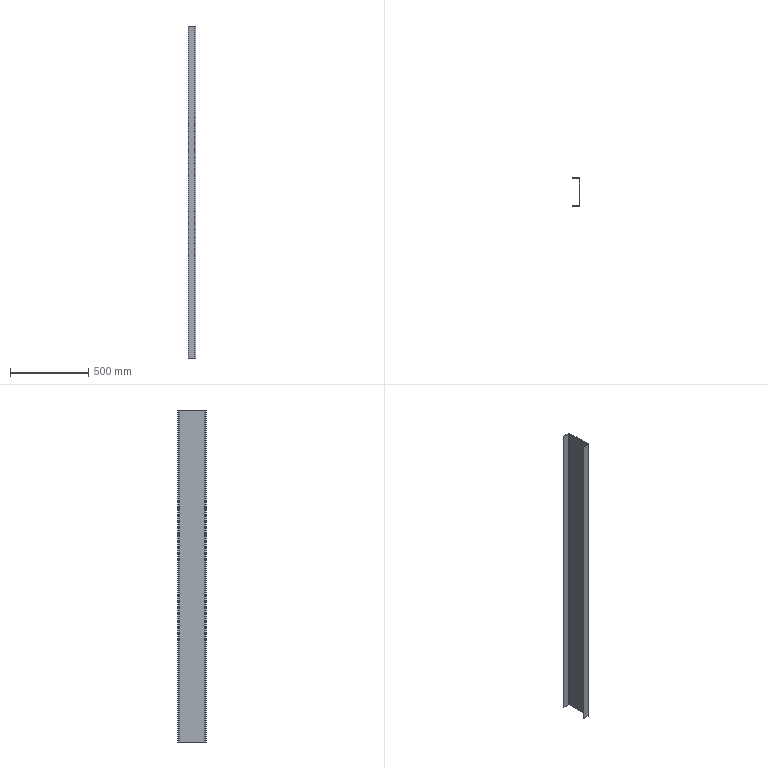Part | SolidWorks | features Extrusion 1 | 1 solid | 14 faces | box 50 x 180 x 2124 mm | volume 2267154 mm3 | plane 10 | cylinder 4 | commonest cylinder face diameters 8 x2 16 x2
STEP:
#1=CARTESIAN_POINT('',(-50.,-86.,-1062.));
#2=VERTEX_POINT('',#1);
#3=CARTESIAN_POINT('',(-50.,-90.,-1062.));
#4=VERTEX_POINT('',#3);
#5=CARTESIAN_POINT('',(-50.,-86.,-1062.));
#6=DIRECTION('',(0.,-1.,0.));
#7=VECTOR('',#6,1000.);
#8=LINE('',#5,#7);
#9=EDGE_CURVE('',#2,#4,#8,.T.);
#10=ORIENTED_EDGE('',*,*,#9,.T.);
#11=CARTESIAN_POINT('',(-50.,-90.,1062.));
#12=VERTEX_POINT('',#11);
#13=CARTESIAN_POINT('',(-50.,-90.,1062.));
#14=DIRECTION('',(0.,0.,-1.));
#15=VECTOR('',#14,1000.);
#16=LINE('',#13,#15);
#17=EDGE_CURVE('',#12,#4,#16,.T.);
#18=ORIENTED_EDGE('',*,*,#17,.F.);
#19=CARTESIAN_POINT('',(-50.,-86.,1062.));
#20=VERTEX_POINT('',#19);
#21=CARTESIAN_POINT('',(-50.,-86.,1062.));
#22=DIRECTION('',(0.,-1.,0.));
#23=VECTOR('',#22,1000.);
#24=LINE('',#21,#23);
#25=EDGE_CURVE('',#20,#12,#24,.T.);
#26=ORIENTED_EDGE('',*,*,#25,.F.);
#27=CARTESIAN_POINT('',(-50.,-86.,1062.));
#28=DIRECTION('',(0.,0.,-1.));
#29=VECTOR('',#28,1000.);
#30=LINE('',#27,#29);
#31=EDGE_CURVE('',#20,#2,#30,.T.);
#32=ORIENTED_EDGE('',*,*,#31,.T.);
#33=EDGE_LOOP('',(#10,#18,#26,#32));
#34=FACE_OUTER_BOUND('',#33,.T.);
#35=CARTESIAN_POINT('',(-50.,-86.,1062.));
#36=DIRECTION('',(1.,0.,0.));
#37=DIRECTION('',(0.,0.,-1.));
#38=AXIS2_PLACEMENT_3D('',#35,#36,#37);
#39=PLANE('',#38);
#40=ADVANCED_FACE('',(#34),#39,.F.);
#41=CARTESIAN_POINT('',(-8.,-90.,-1062.));
#42=VERTEX_POINT('',#41);
#43=CARTESIAN_POINT('',(-50.,-90.,-1062.));
#44=DIRECTION('',(1.,0.,0.));
#45=VECTOR('',#44,1000.);
#46=LINE('',#43,#45);
#47=EDGE_CURVE('',#4,#42,#46,.T.);
#48=ORIENTED_EDGE('',*,*,#47,.T.);
#49=CARTESIAN_POINT('',(-8.,-90.,1062.));
#50=VERTEX_POINT('',#49);
#51=CARTESIAN_POINT('',(-8.,-90.,1062.));
#52=DIRECTION('',(0.,0.,-1.));
#53=VECTOR('',#52,1000.);
#54=LINE('',#51,#53);
#55=EDGE_CURVE('',#50,#42,#54,.T.);
#56=ORIENTED_EDGE('',*,*,#55,.F.);
#57=CARTESIAN_POINT('',(-50.,-90.,1062.));
#58=DIRECTION('',(1.,0.,0.));
#59=VECTOR('',#58,1000.);
#60=LINE('',#57,#59);
#61=EDGE_CURVE('',#12,#50,#60,.T.);
#62=ORIENTED_EDGE('',*,*,#61,.F.);
#63=ORIENTED_EDGE('',*,*,#17,.T.);
#64=EDGE_LOOP('',(#48,#56,#62,#63));
#65=FACE_OUTER_BOUND('',#64,.T.);
#66=CARTESIAN_POINT('',(-50.,-90.,1062.));
#67=DIRECTION('',(0.,1.,0.));
#68=DIRECTION('',(0.,0.,1.));
#69=AXIS2_PLACEMENT_3D('',#66,#67,#68);
#70=PLANE('',#69);
#71=ADVANCED_FACE('',(#65),#70,.F.);
#72=CARTESIAN_POINT('',(0.,-82.,-1062.));
#73=VERTEX_POINT('',#72);
#74=CARTESIAN_POINT('',(-8.,-82.,-1062.));
#75=DIRECTION('',(0.,0.,1.));
#76=DIRECTION('',(1.,0.,0.));
#77=AXIS2_PLACEMENT_3D('',#74,#75,#76);
#78=CIRCLE('',#77,8.);
#79=EDGE_CURVE('',#42,#73,#78,.T.);
#80=ORIENTED_EDGE('',*,*,#79,.T.);
#81=CARTESIAN_POINT('',(0.,-82.,1062.));
#82=VERTEX_POINT('',#81);
#83=CARTESIAN_POINT('',(0.,-82.,1062.));
#84=DIRECTION('',(0.,0.,-1.));
#85=VECTOR('',#84,1000.);
#86=LINE('',#83,#85);
#87=EDGE_CURVE('',#82,#73,#86,.T.);
#88=ORIENTED_EDGE('',*,*,#87,.F.);
#89=CARTESIAN_POINT('',(-8.,-82.,1062.));
#90=DIRECTION('',(0.,0.,1.));
#91=DIRECTION('',(1.,0.,0.));
#92=AXIS2_PLACEMENT_3D('',#89,#90,#91);
#93=CIRCLE('',#92,8.);
#94=EDGE_CURVE('',#50,#82,#93,.T.);
#95=ORIENTED_EDGE('',*,*,#94,.F.);
#96=ORIENTED_EDGE('',*,*,#55,.T.);
#97=EDGE_LOOP('',(#80,#88,#95,#96));
#98=FACE_OUTER_BOUND('',#97,.T.);
#99=CARTESIAN_POINT('',(-8.,-82.,1062.));
#100=DIRECTION('',(0.,0.,-1.));
#101=DIRECTION('',(-1.,0.,0.));
#102=AXIS2_PLACEMENT_3D('',#99,#100,#101);
#103=CYLINDRICAL_SURFACE('',#102,8.);
#104=ADVANCED_FACE('',(#98),#103,.T.);
#105=CARTESIAN_POINT('',(0.,82.,-1062.));
#106=VERTEX_POINT('',#105);
#107=CARTESIAN_POINT('',(0.,-82.,-1062.));
#108=DIRECTION('',(0.,1.,0.));
#109=VECTOR('',#108,1000.);
#110=LINE('',#107,#109);
#111=EDGE_CURVE('',#73,#106,#110,.T.);
#112=ORIENTED_EDGE('',*,*,#111,.T.);
#113=CARTESIAN_POINT('',(0.,82.,1062.));
#114=VERTEX_POINT('',#113);
#115=CARTESIAN_POINT('',(0.,82.,1062.));
#116=DIRECTION('',(0.,0.,-1.));
#117=VECTOR('',#116,1000.);
#118=LINE('',#115,#117);
#119=EDGE_CURVE('',#114,#106,#118,.T.);
#120=ORIENTED_EDGE('',*,*,#119,.F.);
#121=CARTESIAN_POINT('',(0.,-82.,1062.));
#122=DIRECTION('',(0.,1.,0.));
#123=VECTOR('',#122,1000.);
#124=LINE('',#121,#123);
#125=EDGE_CURVE('',#82,#114,#124,.T.);
#126=ORIENTED_EDGE('',*,*,#125,.F.);
#127=ORIENTED_EDGE('',*,*,#87,.T.);
#128=EDGE_LOOP('',(#112,#120,#126,#127));
#129=FACE_OUTER_BOUND('',#128,.T.);
#130=CARTESIAN_POINT('',(0.,-82.,1062.));
#131=DIRECTION('',(-1.,0.,0.));
#132=DIRECTION('',(0.,0.,1.));
#133=AXIS2_PLACEMENT_3D('',#130,#131,#132);
#134=PLANE('',#133);
#135=ADVANCED_FACE('',(#129),#134,.F.);
#136=CARTESIAN_POINT('',(-8.,90.,-1062.));
#137=VERTEX_POINT('',#136);
#138=CARTESIAN_POINT('',(-8.,82.,-1062.));
#139=DIRECTION('',(0.,0.,1.));
#140=DIRECTION('',(1.,0.,0.));
#141=AXIS2_PLACEMENT_3D('',#138,#139,#140);
#142=CIRCLE('',#141,8.);
#143=EDGE_CURVE('',#106,#137,#142,.T.);
#144=ORIENTED_EDGE('',*,*,#143,.T.);
#145=CARTESIAN_POINT('',(-8.,90.,1062.));
#146=VERTEX_POINT('',#145);
#147=CARTESIAN_POINT('',(-8.,90.,1062.));
#148=DIRECTION('',(0.,0.,-1.));
#149=VECTOR('',#148,1000.);
#150=LINE('',#147,#149);
#151=EDGE_CURVE('',#146,#137,#150,.T.);
#152=ORIENTED_EDGE('',*,*,#151,.F.);
#153=CARTESIAN_POINT('',(-8.,82.,1062.));
#154=DIRECTION('',(0.,0.,1.));
#155=DIRECTION('',(1.,0.,0.));
#156=AXIS2_PLACEMENT_3D('',#153,#154,#155);
#157=CIRCLE('',#156,8.);
#158=EDGE_CURVE('',#114,#146,#157,.T.);
#159=ORIENTED_EDGE('',*,*,#158,.F.);
#160=ORIENTED_EDGE('',*,*,#119,.T.);
#161=EDGE_LOOP('',(#144,#152,#159,#160));
#162=FACE_OUTER_BOUND('',#161,.T.);
#163=CARTESIAN_POINT('',(-8.,82.,1062.));
#164=DIRECTION('',(0.,0.,-1.));
#165=DIRECTION('',(-1.,0.,0.));
#166=AXIS2_PLACEMENT_3D('',#163,#164,#165);
#167=CYLINDRICAL_SURFACE('',#166,8.);
#168=ADVANCED_FACE('',(#162),#167,.T.);
#169=CARTESIAN_POINT('',(-50.,90.,-1062.));
#170=VERTEX_POINT('',#169);
#171=CARTESIAN_POINT('',(-8.,90.,-1062.));
#172=DIRECTION('',(-1.,0.,0.));
#173=VECTOR('',#172,1000.);
#174=LINE('',#171,#173);
#175=EDGE_CURVE('',#137,#170,#174,.T.);
#176=ORIENTED_EDGE('',*,*,#175,.T.);
#177=CARTESIAN_POINT('',(-50.,90.,1062.));
#178=VERTEX_POINT('',#177);
#179=CARTESIAN_POINT('',(-50.,90.,1062.));
#180=DIRECTION('',(0.,0.,-1.));
#181=VECTOR('',#180,1000.);
#182=LINE('',#179,#181);
#183=EDGE_CURVE('',#178,#170,#182,.T.);
#184=ORIENTED_EDGE('',*,*,#183,.F.);
#185=CARTESIAN_POINT('',(-8.,90.,1062.));
#186=DIRECTION('',(-1.,0.,0.));
#187=VECTOR('',#186,1000.);
#188=LINE('',#185,#187);
#189=EDGE_CURVE('',#146,#178,#188,.T.);
#190=ORIENTED_EDGE('',*,*,#189,.F.);
#191=ORIENTED_EDGE('',*,*,#151,.T.);
#192=EDGE_LOOP('',(#176,#184,#190,#191));
#193=FACE_OUTER_BOUND('',#192,.T.);
#194=CARTESIAN_POINT('',(-8.,90.,1062.));
#195=DIRECTION('',(0.,-1.,0.));
#196=DIRECTION('',(0.,0.,-1.));
#197=AXIS2_PLACEMENT_3D('',#194,#195,#196);
#198=PLANE('',#197);
#199=ADVANCED_FACE('',(#193),#198,.F.);
#200=CARTESIAN_POINT('',(-50.,86.,-1062.));
#201=VERTEX_POINT('',#200);
#202=CARTESIAN_POINT('',(-50.,90.,-1062.));
#203=DIRECTION('',(0.,-1.,0.));
#204=VECTOR('',#203,1000.);
#205=LINE('',#202,#204);
#206=EDGE_CURVE('',#170,#201,#205,.T.);
#207=ORIENTED_EDGE('',*,*,#206,.T.);
#208=CARTESIAN_POINT('',(-50.,86.,1062.));
#209=VERTEX_POINT('',#208);
#210=CARTESIAN_POINT('',(-50.,86.,1062.));
#211=DIRECTION('',(0.,0.,-1.));
#212=VECTOR('',#211,1000.);
#213=LINE('',#210,#212);
#214=EDGE_CURVE('',#209,#201,#213,.T.);
#215=ORIENTED_EDGE('',*,*,#214,.F.);
#216=CARTESIAN_POINT('',(-50.,90.,1062.));
#217=DIRECTION('',(0.,-1.,0.));
#218=VECTOR('',#217,1000.);
#219=LINE('',#216,#218);
#220=EDGE_CURVE('',#178,#209,#219,.T.);
#221=ORIENTED_EDGE('',*,*,#220,.F.);
#222=ORIENTED_EDGE('',*,*,#183,.T.);
#223=EDGE_LOOP('',(#207,#215,#221,#222));
#224=FACE_OUTER_BOUND('',#223,.T.);
#225=CARTESIAN_POINT('',(-50.,90.,1062.));
#226=DIRECTION('',(1.,0.,0.));
#227=DIRECTION('',(0.,0.,-1.));
#228=AXIS2_PLACEMENT_3D('',#225,#226,#227);
#229=PLANE('',#228);
#230=ADVANCED_FACE('',(#224),#229,.F.);
#231=CARTESIAN_POINT('',(-8.,86.,-1062.));
#232=VERTEX_POINT('',#231);
#233=CARTESIAN_POINT('',(-50.,86.,-1062.));
#234=DIRECTION('',(1.,0.,0.));
#235=VECTOR('',#234,1000.);
#236=LINE('',#233,#235);
#237=EDGE_CURVE('',#201,#232,#236,.T.);
#238=ORIENTED_EDGE('',*,*,#237,.T.);
#239=CARTESIAN_POINT('',(-8.,86.,1062.));
#240=VERTEX_POINT('',#239);
#241=CARTESIAN_POINT('',(-8.,86.,1062.));
#242=DIRECTION('',(0.,0.,-1.));
#243=VECTOR('',#242,1000.);
#244=LINE('',#241,#243);
#245=EDGE_CURVE('',#240,#232,#244,.T.);
#246=ORIENTED_EDGE('',*,*,#245,.F.);
#247=CARTESIAN_POINT('',(-50.,86.,1062.));
#248=DIRECTION('',(1.,0.,0.));
#249=VECTOR('',#248,1000.);
#250=LINE('',#247,#249);
#251=EDGE_CURVE('',#209,#240,#250,.T.);
#252=ORIENTED_EDGE('',*,*,#251,.F.);
#253=ORIENTED_EDGE('',*,*,#214,.T.);
#254=EDGE_LOOP('',(#238,#246,#252,#253));
#255=FACE_OUTER_BOUND('',#254,.T.);
#256=CARTESIAN_POINT('',(-50.,86.,1062.));
#257=DIRECTION('',(0.,1.,0.));
#258=DIRECTION('',(0.,0.,1.));
#259=AXIS2_PLACEMENT_3D('',#256,#257,#258);
#260=PLANE('',#259);
#261=ADVANCED_FACE('',(#255),#260,.F.);
#262=CARTESIAN_POINT('',(-4.,82.,-1062.));
#263=VERTEX_POINT('',#262);
#264=CARTESIAN_POINT('',(-8.,82.,-1062.));
#265=DIRECTION('',(0.,0.,-1.));
#266=DIRECTION('',(1.,0.,0.));
#267=AXIS2_PLACEMENT_3D('',#264,#265,#266);
#268=CIRCLE('',#267,4.);
#269=EDGE_CURVE('',#232,#263,#268,.T.);
#270=ORIENTED_EDGE('',*,*,#269,.T.);
#271=CARTESIAN_POINT('',(-4.,82.,1062.));
#272=VERTEX_POINT('',#271);
#273=CARTESIAN_POINT('',(-4.,82.,1062.));
#274=DIRECTION('',(0.,0.,-1.));
#275=VECTOR('',#274,1000.);
#276=LINE('',#273,#275);
#277=EDGE_CURVE('',#272,#263,#276,.T.);
#278=ORIENTED_EDGE('',*,*,#277,.F.);
#279=CARTESIAN_POINT('',(-8.,82.,1062.));
#280=DIRECTION('',(0.,0.,-1.));
#281=DIRECTION('',(1.,0.,0.));
#282=AXIS2_PLACEMENT_3D('',#279,#280,#281);
#283=CIRCLE('',#282,4.);
#284=EDGE_CURVE('',#240,#272,#283,.T.);
#285=ORIENTED_EDGE('',*,*,#284,.F.);
#286=ORIENTED_EDGE('',*,*,#245,.T.);
#287=EDGE_LOOP('',(#270,#278,#285,#286));
#288=FACE_OUTER_BOUND('',#287,.T.);
#289=CARTESIAN_POINT('',(-8.,82.,1062.));
#290=DIRECTION('',(0.,0.,-1.));
#291=DIRECTION('',(-1.,0.,0.));
#292=AXIS2_PLACEMENT_3D('',#289,#290,#291);
#293=CYLINDRICAL_SURFACE('',#292,4.);
#294=ADVANCED_FACE('',(#288),#293,.F.);
#295=CARTESIAN_POINT('',(-4.,-82.,-1062.));
#296=VERTEX_POINT('',#295);
#297=CARTESIAN_POINT('',(-4.,82.,-1062.));
#298=DIRECTION('',(0.,-1.,0.));
#299=VECTOR('',#298,1000.);
#300=LINE('',#297,#299);
#301=EDGE_CURVE('',#263,#296,#300,.T.);
#302=ORIENTED_EDGE('',*,*,#301,.T.);
#303=CARTESIAN_POINT('',(-4.,-82.,1062.));
#304=VERTEX_POINT('',#303);
#305=CARTESIAN_POINT('',(-4.,-82.,1062.));
#306=DIRECTION('',(0.,0.,-1.));
#307=VECTOR('',#306,1000.);
#308=LINE('',#305,#307);
#309=EDGE_CURVE('',#304,#296,#308,.T.);
#310=ORIENTED_EDGE('',*,*,#309,.F.);
#311=CARTESIAN_POINT('',(-4.,82.,1062.));
#312=DIRECTION('',(0.,-1.,0.));
#313=VECTOR('',#312,1000.);
#314=LINE('',#311,#313);
#315=EDGE_CURVE('',#272,#304,#314,.T.);
#316=ORIENTED_EDGE('',*,*,#315,.F.);
#317=ORIENTED_EDGE('',*,*,#277,.T.);
#318=EDGE_LOOP('',(#302,#310,#316,#317));
#319=FACE_OUTER_BOUND('',#318,.T.);
#320=CARTESIAN_POINT('',(-4.,82.,1062.));
#321=DIRECTION('',(1.,0.,0.));
#322=DIRECTION('',(0.,1.,0.));
#323=AXIS2_PLACEMENT_3D('',#320,#321,#322);
#324=PLANE('',#323);
#325=ADVANCED_FACE('',(#319),#324,.F.);
#326=CARTESIAN_POINT('',(-8.,-86.,-1062.));
#327=VERTEX_POINT('',#326);
#328=CARTESIAN_POINT('',(-8.,-82.,-1062.));
#329=DIRECTION('',(0.,0.,-1.));
#330=DIRECTION('',(1.,0.,0.));
#331=AXIS2_PLACEMENT_3D('',#328,#329,#330);
#332=CIRCLE('',#331,4.);
#333=EDGE_CURVE('',#296,#327,#332,.T.);
#334=ORIENTED_EDGE('',*,*,#333,.T.);
#335=CARTESIAN_POINT('',(-8.,-86.,1062.));
#336=VERTEX_POINT('',#335);
#337=CARTESIAN_POINT('',(-8.,-86.,1062.));
#338=DIRECTION('',(0.,0.,-1.));
#339=VECTOR('',#338,1000.);
#340=LINE('',#337,#339);
#341=EDGE_CURVE('',#336,#327,#340,.T.);
#342=ORIENTED_EDGE('',*,*,#341,.F.);
#343=CARTESIAN_POINT('',(-8.,-82.,1062.));
#344=DIRECTION('',(0.,0.,-1.));
#345=DIRECTION('',(1.,0.,0.));
#346=AXIS2_PLACEMENT_3D('',#343,#344,#345);
#347=CIRCLE('',#346,4.);
#348=EDGE_CURVE('',#304,#336,#347,.T.);
#349=ORIENTED_EDGE('',*,*,#348,.F.);
#350=ORIENTED_EDGE('',*,*,#309,.T.);
#351=EDGE_LOOP('',(#334,#342,#349,#350));
#352=FACE_OUTER_BOUND('',#351,.T.);
#353=CARTESIAN_POINT('',(-8.,-82.,1062.));
#354=DIRECTION('',(0.,0.,-1.));
#355=DIRECTION('',(-1.,0.,0.));
#356=AXIS2_PLACEMENT_3D('',#353,#354,#355);
#357=CYLINDRICAL_SURFACE('',#356,4.);
#358=ADVANCED_FACE('',(#352),#357,.F.);
#359=CARTESIAN_POINT('',(-8.,-86.,-1062.));
#360=DIRECTION('',(-1.,0.,0.));
#361=VECTOR('',#360,1000.);
#362=LINE('',#359,#361);
#363=EDGE_CURVE('',#327,#2,#362,.T.);
#364=ORIENTED_EDGE('',*,*,#363,.T.);
#365=ORIENTED_EDGE('',*,*,#31,.F.);
#366=CARTESIAN_POINT('',(-8.,-86.,1062.));
#367=DIRECTION('',(-1.,0.,0.));
#368=VECTOR('',#367,1000.);
#369=LINE('',#366,#368);
#370=EDGE_CURVE('',#336,#20,#369,.T.);
#371=ORIENTED_EDGE('',*,*,#370,.F.);
#372=ORIENTED_EDGE('',*,*,#341,.T.);
#373=EDGE_LOOP('',(#364,#365,#371,#372));
#374=FACE_OUTER_BOUND('',#373,.T.);
#375=CARTESIAN_POINT('',(-8.,-86.,1062.));
#376=DIRECTION('',(0.,-1.,0.));
#377=DIRECTION('',(0.,0.,-1.));
#378=AXIS2_PLACEMENT_3D('',#375,#376,#377);
#379=PLANE('',#378);
#380=ADVANCED_FACE('',(#374),#379,.F.);
#381=ORIENTED_EDGE('',*,*,#25,.T.);
#382=ORIENTED_EDGE('',*,*,#61,.T.);
#383=ORIENTED_EDGE('',*,*,#94,.T.);
#384=ORIENTED_EDGE('',*,*,#125,.T.);
#385=ORIENTED_EDGE('',*,*,#158,.T.);
#386=ORIENTED_EDGE('',*,*,#189,.T.);
#387=ORIENTED_EDGE('',*,*,#220,.T.);
#388=ORIENTED_EDGE('',*,*,#251,.T.);
#389=ORIENTED_EDGE('',*,*,#284,.T.);
#390=ORIENTED_EDGE('',*,*,#315,.T.);
#391=ORIENTED_EDGE('',*,*,#348,.T.);
#392=ORIENTED_EDGE('',*,*,#370,.T.);
#393=EDGE_LOOP('',(#381,#382,#383,#384,#385,#386,#387,#388,#389,#390,#391,#392));
#394=FACE_OUTER_BOUND('',#393,.T.);
#395=CARTESIAN_POINT('',(-8.,-82.,1062.));
#396=DIRECTION('',(0.,0.,1.));
#397=DIRECTION('',(1.,0.,0.));
#398=AXIS2_PLACEMENT_3D('',#395,#396,#397);
#399=PLANE('',#398);
#400=ADVANCED_FACE('',(#394),#399,.T.);
#401=ORIENTED_EDGE('',*,*,#9,.F.);
#402=ORIENTED_EDGE('',*,*,#363,.F.);
#403=ORIENTED_EDGE('',*,*,#333,.F.);
#404=ORIENTED_EDGE('',*,*,#301,.F.);
#405=ORIENTED_EDGE('',*,*,#269,.F.);
#406=ORIENTED_EDGE('',*,*,#237,.F.);
#407=ORIENTED_EDGE('',*,*,#206,.F.);
#408=ORIENTED_EDGE('',*,*,#175,.F.);
#409=ORIENTED_EDGE('',*,*,#143,.F.);
#410=ORIENTED_EDGE('',*,*,#111,.F.);
#411=ORIENTED_EDGE('',*,*,#79,.F.);
#412=ORIENTED_EDGE('',*,*,#47,.F.);
#413=EDGE_LOOP('',(#401,#402,#403,#404,#405,#406,#407,#408,#409,#410,#411,#412));
#414=FACE_OUTER_BOUND('',#413,.T.);
#415=CARTESIAN_POINT('',(-8.,-82.,-1062.));
#416=DIRECTION('',(0.,0.,1.));
#417=DIRECTION('',(1.,0.,0.));
#418=AXIS2_PLACEMENT_3D('',#415,#416,#417);
#419=PLANE('',#418);
#420=ADVANCED_FACE('',(#414),#419,.F.);
#421=CLOSED_SHELL('',(#40,#71,#104,#135,#168,#199,#230,#261,#294,#325,#358,#380,#400,#420));
#422=MANIFOLD_SOLID_BREP('',#421);
#423=CARTESIAN_POINT('',(0.,0.,0.));
#424=DIRECTION('',(0.,0.,1.));
#425=DIRECTION('',(1.,0.,0.));
#426=AXIS2_PLACEMENT_3D('',#423,#424,#425);
#427=(LENGTH_UNIT()NAMED_UNIT(*)SI_UNIT(.MILLI.,.METRE.));
#428=UNCERTAINTY_MEASURE_WITH_UNIT(LENGTH_MEASURE(0.00001),#427,'','');
#429=(NAMED_UNIT(*)PLANE_ANGLE_UNIT()SI_UNIT($,.RADIAN.));
#430=(NAMED_UNIT(*)SI_UNIT($,.STERADIAN.)SOLID_ANGLE_UNIT());
#431=(GEOMETRIC_REPRESENTATION_CONTEXT(3)GLOBAL_UNCERTAINTY_ASSIGNED_CONTEXT((#428))GLOBAL_UNIT_ASSIGNED_CONTEXT((#427,#429,#430))REPRESENTATION_CONTEXT('',''));
#432=ADVANCED_BREP_SHAPE_REPRESENTATION('',(#422,#426),#431);